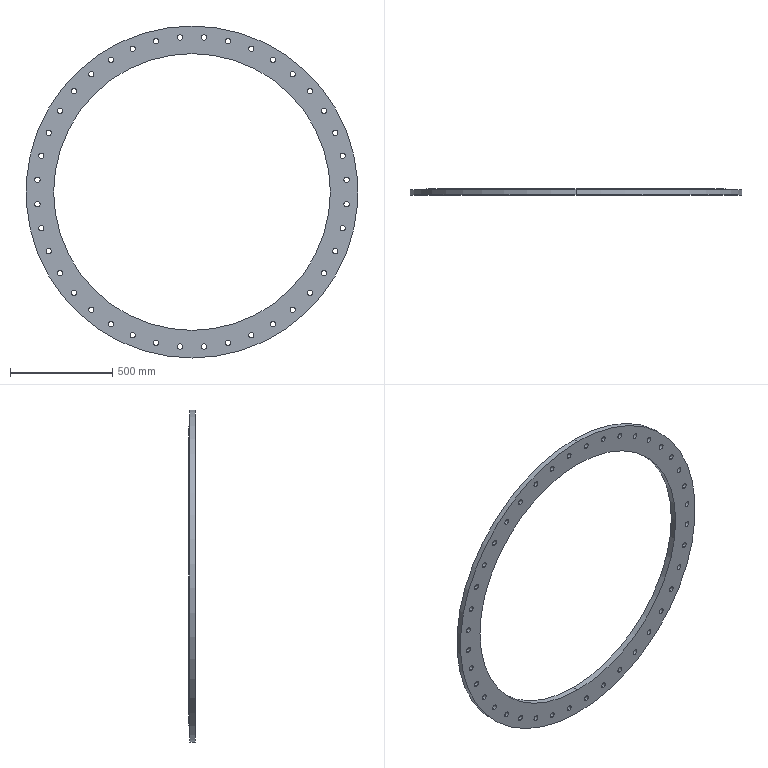Part | SolidWorks | features ICE 4, HoleWzd 2, Extrusion 1 | 1 solid | 89 faces | box 1620 x 30 x 1620 mm | volume 16428173 mm3 | cylinder 86 | plane 3 | commonest cylinder face diameters 26 x80 1350 x2 1460 x2 1620 x2